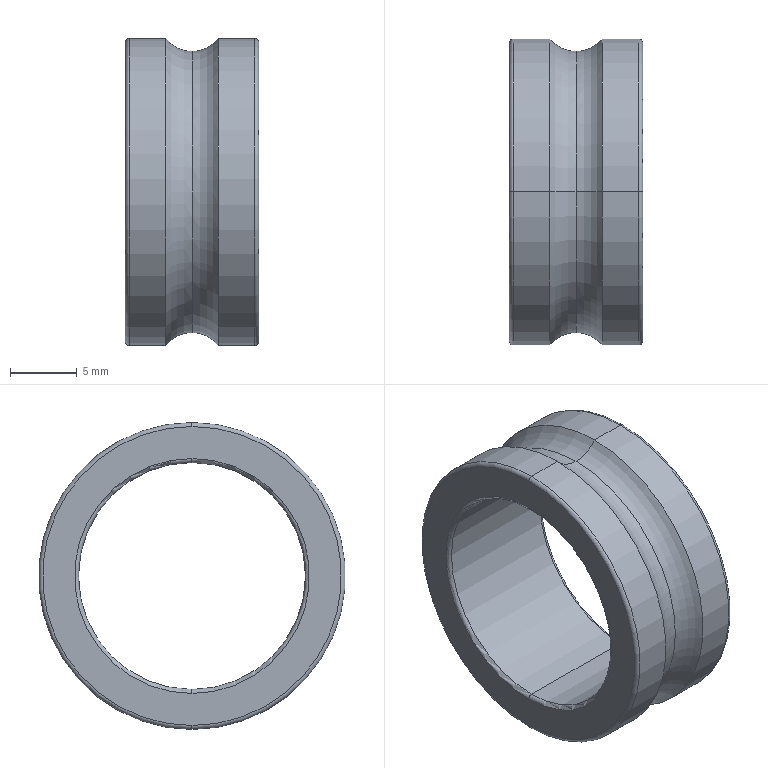Part | SolidWorks | features BaseBody 1 | 1 solid | 20 faces | box 10 x 23 x 23 mm | volume 1693 mm3 | torus 12 | cylinder 6 | plane 2 | commonest cylinder face diameters 23 x4 17 x2
STEP:
#1=CARTESIAN_POINT('',(-1.969,0.,11.5));
#2=VERTEX_POINT('',#1);
#3=CARTESIAN_POINT('',(0.,0.,10.525));
#4=VERTEX_POINT('',#3);
#5=CARTESIAN_POINT('',(0.,0.,13.));
#6=DIRECTION('',(0.,-1.,0.));
#7=DIRECTION('',(0.,0.,-1.));
#8=AXIS2_PLACEMENT_3D('',#5,#6,#7);
#9=CIRCLE('',#8,2.475);
#10=EDGE_CURVE('',#2,#4,#9,.T.);
#11=ORIENTED_EDGE('',*,*,#10,.T.);
#12=CARTESIAN_POINT('',(0.,0.,-10.525));
#13=VERTEX_POINT('',#12);
#14=CARTESIAN_POINT('',(0.,0.,0.));
#15=DIRECTION('',(-1.,0.,0.));
#16=DIRECTION('',(0.,0.,1.));
#17=AXIS2_PLACEMENT_3D('',#14,#15,#16);
#18=CIRCLE('',#17,10.525);
#19=EDGE_CURVE('',#4,#13,#18,.T.);
#20=ORIENTED_EDGE('',*,*,#19,.T.);
#21=CARTESIAN_POINT('',(-1.969,0.,-11.5));
#22=VERTEX_POINT('',#21);
#23=CARTESIAN_POINT('',(0.,0.,-13.));
#24=DIRECTION('',(0.,1.,0.));
#25=DIRECTION('',(0.,0.,1.));
#26=AXIS2_PLACEMENT_3D('',#23,#24,#25);
#27=CIRCLE('',#26,2.475);
#28=EDGE_CURVE('',#22,#13,#27,.T.);
#29=ORIENTED_EDGE('',*,*,#28,.F.);
#30=CARTESIAN_POINT('',(-1.969,0.,0.));
#31=DIRECTION('',(1.,0.,0.));
#32=DIRECTION('',(0.,0.,-1.));
#33=AXIS2_PLACEMENT_3D('',#30,#31,#32);
#34=CIRCLE('',#33,11.5);
#35=EDGE_CURVE('',#22,#2,#34,.T.);
#36=ORIENTED_EDGE('',*,*,#35,.T.);
#37=EDGE_LOOP('',(#11,#20,#29,#36));
#38=FACE_OUTER_BOUND('',#37,.T.);
#39=CARTESIAN_POINT('',(0.,0.,0.));
#40=DIRECTION('',(-1.,0.,0.));
#41=DIRECTION('',(0.,0.,1.));
#42=AXIS2_PLACEMENT_3D('',#39,#40,#41);
#43=TOROIDAL_SURFACE('',#42,13.,2.475);
#44=ADVANCED_FACE('',(#38),#43,.F.);
#45=ORIENTED_EDGE('',*,*,#28,.T.);
#46=CARTESIAN_POINT('',(0.,0.,0.));
#47=DIRECTION('',(-1.,0.,0.));
#48=DIRECTION('',(0.,0.,1.));
#49=AXIS2_PLACEMENT_3D('',#46,#47,#48);
#50=CIRCLE('',#49,10.525);
#51=EDGE_CURVE('',#13,#4,#50,.T.);
#52=ORIENTED_EDGE('',*,*,#51,.T.);
#53=ORIENTED_EDGE('',*,*,#10,.F.);
#54=CARTESIAN_POINT('',(-1.969,0.,0.));
#55=DIRECTION('',(1.,0.,0.));
#56=DIRECTION('',(0.,0.,-1.));
#57=AXIS2_PLACEMENT_3D('',#54,#55,#56);
#58=CIRCLE('',#57,11.5);
#59=EDGE_CURVE('',#2,#22,#58,.T.);
#60=ORIENTED_EDGE('',*,*,#59,.T.);
#61=EDGE_LOOP('',(#45,#52,#53,#60));
#62=FACE_OUTER_BOUND('',#61,.T.);
#63=CARTESIAN_POINT('',(0.,0.,0.));
#64=DIRECTION('',(-1.,0.,0.));
#65=DIRECTION('',(0.,0.,1.));
#66=AXIS2_PLACEMENT_3D('',#63,#64,#65);
#67=TOROIDAL_SURFACE('',#66,13.,2.475);
#68=ADVANCED_FACE('',(#62),#67,.F.);
#69=ORIENTED_EDGE('',*,*,#51,.F.);
#70=CARTESIAN_POINT('',(1.969,0.,-11.5));
#71=VERTEX_POINT('',#70);
#72=CARTESIAN_POINT('',(0.,0.,-13.));
#73=DIRECTION('',(0.,1.,0.));
#74=DIRECTION('',(0.,0.,1.));
#75=AXIS2_PLACEMENT_3D('',#72,#73,#74);
#76=CIRCLE('',#75,2.475);
#77=EDGE_CURVE('',#13,#71,#76,.T.);
#78=ORIENTED_EDGE('',*,*,#77,.T.);
#79=CARTESIAN_POINT('',(1.969,0.,11.5));
#80=VERTEX_POINT('',#79);
#81=CARTESIAN_POINT('',(1.969,0.,0.));
#82=DIRECTION('',(-1.,0.,0.));
#83=DIRECTION('',(0.,0.,1.));
#84=AXIS2_PLACEMENT_3D('',#81,#82,#83);
#85=CIRCLE('',#84,11.5);
#86=EDGE_CURVE('',#71,#80,#85,.T.);
#87=ORIENTED_EDGE('',*,*,#86,.T.);
#88=CARTESIAN_POINT('',(0.,0.,13.));
#89=DIRECTION('',(0.,-1.,0.));
#90=DIRECTION('',(0.,0.,-1.));
#91=AXIS2_PLACEMENT_3D('',#88,#89,#90);
#92=CIRCLE('',#91,2.475);
#93=EDGE_CURVE('',#4,#80,#92,.T.);
#94=ORIENTED_EDGE('',*,*,#93,.F.);
#95=EDGE_LOOP('',(#69,#78,#87,#94));
#96=FACE_OUTER_BOUND('',#95,.T.);
#97=CARTESIAN_POINT('',(0.,0.,0.));
#98=DIRECTION('',(-1.,0.,0.));
#99=DIRECTION('',(0.,0.,1.));
#100=AXIS2_PLACEMENT_3D('',#97,#98,#99);
#101=TOROIDAL_SURFACE('',#100,13.,2.475);
#102=ADVANCED_FACE('',(#96),#101,.F.);
#103=CARTESIAN_POINT('',(-4.7,0.,11.5));
#104=VERTEX_POINT('',#103);
#105=CARTESIAN_POINT('',(-4.7,0.,-11.5));
#106=VERTEX_POINT('',#105);
#107=CARTESIAN_POINT('',(-4.7,0.,0.));
#108=DIRECTION('',(-1.,0.,0.));
#109=DIRECTION('',(0.,0.,1.));
#110=AXIS2_PLACEMENT_3D('',#107,#108,#109);
#111=CIRCLE('',#110,11.5);
#112=EDGE_CURVE('',#104,#106,#111,.T.);
#113=ORIENTED_EDGE('',*,*,#112,.T.);
#114=CARTESIAN_POINT('',(-5.,0.,-11.2));
#115=VERTEX_POINT('',#114);
#116=CARTESIAN_POINT('',(-4.7,0.,-11.2));
#117=DIRECTION('',(0.,1.,0.));
#118=DIRECTION('',(0.,0.,1.));
#119=AXIS2_PLACEMENT_3D('',#116,#117,#118);
#120=CIRCLE('',#119,0.3);
#121=EDGE_CURVE('',#106,#115,#120,.T.);
#122=ORIENTED_EDGE('',*,*,#121,.T.);
#123=CARTESIAN_POINT('',(-5.,0.,11.2));
#124=VERTEX_POINT('',#123);
#125=CARTESIAN_POINT('',(-5.,0.,0.));
#126=DIRECTION('',(-1.,0.,0.));
#127=DIRECTION('',(0.,0.,1.));
#128=AXIS2_PLACEMENT_3D('',#125,#126,#127);
#129=CIRCLE('',#128,11.2);
#130=EDGE_CURVE('',#124,#115,#129,.T.);
#131=ORIENTED_EDGE('',*,*,#130,.F.);
#132=CARTESIAN_POINT('',(-4.7,0.,11.2));
#133=DIRECTION('',(0.,-1.,0.));
#134=DIRECTION('',(0.,0.,-1.));
#135=AXIS2_PLACEMENT_3D('',#132,#133,#134);
#136=CIRCLE('',#135,0.3);
#137=EDGE_CURVE('',#104,#124,#136,.T.);
#138=ORIENTED_EDGE('',*,*,#137,.F.);
#139=EDGE_LOOP('',(#113,#122,#131,#138));
#140=FACE_OUTER_BOUND('',#139,.T.);
#141=CARTESIAN_POINT('',(-4.7,0.,0.));
#142=DIRECTION('',(-1.,0.,0.));
#143=DIRECTION('',(0.,0.,1.));
#144=AXIS2_PLACEMENT_3D('',#141,#142,#143);
#145=TOROIDAL_SURFACE('',#144,11.2,0.3);
#146=ADVANCED_FACE('',(#140),#145,.T.);
#147=CARTESIAN_POINT('',(5.,0.,11.2));
#148=VERTEX_POINT('',#147);
#149=CARTESIAN_POINT('',(5.,0.,-11.2));
#150=VERTEX_POINT('',#149);
#151=CARTESIAN_POINT('',(5.,0.,0.));
#152=DIRECTION('',(-1.,0.,0.));
#153=DIRECTION('',(0.,0.,1.));
#154=AXIS2_PLACEMENT_3D('',#151,#152,#153);
#155=CIRCLE('',#154,11.2);
#156=EDGE_CURVE('',#148,#150,#155,.T.);
#157=ORIENTED_EDGE('',*,*,#156,.T.);
#158=CARTESIAN_POINT('',(4.7,0.,-11.5));
#159=VERTEX_POINT('',#158);
#160=CARTESIAN_POINT('',(4.7,0.,-11.2));
#161=DIRECTION('',(0.,1.,0.));
#162=DIRECTION('',(0.,0.,1.));
#163=AXIS2_PLACEMENT_3D('',#160,#161,#162);
#164=CIRCLE('',#163,0.3);
#165=EDGE_CURVE('',#150,#159,#164,.T.);
#166=ORIENTED_EDGE('',*,*,#165,.T.);
#167=CARTESIAN_POINT('',(4.7,0.,11.5));
#168=VERTEX_POINT('',#167);
#169=CARTESIAN_POINT('',(4.7,0.,0.));
#170=DIRECTION('',(-1.,0.,0.));
#171=DIRECTION('',(0.,0.,1.));
#172=AXIS2_PLACEMENT_3D('',#169,#170,#171);
#173=CIRCLE('',#172,11.5);
#174=EDGE_CURVE('',#168,#159,#173,.T.);
#175=ORIENTED_EDGE('',*,*,#174,.F.);
#176=CARTESIAN_POINT('',(4.7,0.,11.2));
#177=DIRECTION('',(0.,-1.,0.));
#178=DIRECTION('',(0.,0.,-1.));
#179=AXIS2_PLACEMENT_3D('',#176,#177,#178);
#180=CIRCLE('',#179,0.3);
#181=EDGE_CURVE('',#148,#168,#180,.T.);
#182=ORIENTED_EDGE('',*,*,#181,.F.);
#183=EDGE_LOOP('',(#157,#166,#175,#182));
#184=FACE_OUTER_BOUND('',#183,.T.);
#185=CARTESIAN_POINT('',(4.7,0.,0.));
#186=DIRECTION('',(-1.,0.,0.));
#187=DIRECTION('',(0.,0.,1.));
#188=AXIS2_PLACEMENT_3D('',#185,#186,#187);
#189=TOROIDAL_SURFACE('',#188,11.2,0.3);
#190=ADVANCED_FACE('',(#184),#189,.T.);
#191=CARTESIAN_POINT('',(4.7,0.,8.5));
#192=VERTEX_POINT('',#191);
#193=CARTESIAN_POINT('',(4.7,0.,-8.5));
#194=VERTEX_POINT('',#193);
#195=CARTESIAN_POINT('',(4.7,0.,0.));
#196=DIRECTION('',(-1.,0.,0.));
#197=DIRECTION('',(0.,0.,1.));
#198=AXIS2_PLACEMENT_3D('',#195,#196,#197);
#199=CIRCLE('',#198,8.5);
#200=EDGE_CURVE('',#192,#194,#199,.T.);
#201=ORIENTED_EDGE('',*,*,#200,.T.);
#202=CARTESIAN_POINT('',(5.,0.,-8.8));
#203=VERTEX_POINT('',#202);
#204=CARTESIAN_POINT('',(4.7,0.,-8.8));
#205=DIRECTION('',(0.,1.,0.));
#206=DIRECTION('',(0.,0.,1.));
#207=AXIS2_PLACEMENT_3D('',#204,#205,#206);
#208=CIRCLE('',#207,0.3);
#209=EDGE_CURVE('',#194,#203,#208,.T.);
#210=ORIENTED_EDGE('',*,*,#209,.T.);
#211=CARTESIAN_POINT('',(5.,0.,8.8));
#212=VERTEX_POINT('',#211);
#213=CARTESIAN_POINT('',(5.,0.,0.));
#214=DIRECTION('',(-1.,0.,0.));
#215=DIRECTION('',(0.,0.,1.));
#216=AXIS2_PLACEMENT_3D('',#213,#214,#215);
#217=CIRCLE('',#216,8.8);
#218=EDGE_CURVE('',#212,#203,#217,.T.);
#219=ORIENTED_EDGE('',*,*,#218,.F.);
#220=CARTESIAN_POINT('',(4.7,0.,8.8));
#221=DIRECTION('',(0.,-1.,0.));
#222=DIRECTION('',(0.,0.,-1.));
#223=AXIS2_PLACEMENT_3D('',#220,#221,#222);
#224=CIRCLE('',#223,0.3);
#225=EDGE_CURVE('',#192,#212,#224,.T.);
#226=ORIENTED_EDGE('',*,*,#225,.F.);
#227=EDGE_LOOP('',(#201,#210,#219,#226));
#228=FACE_OUTER_BOUND('',#227,.T.);
#229=CARTESIAN_POINT('',(4.7,0.,0.));
#230=DIRECTION('',(-1.,0.,0.));
#231=DIRECTION('',(0.,0.,1.));
#232=AXIS2_PLACEMENT_3D('',#229,#230,#231);
#233=TOROIDAL_SURFACE('',#232,8.8,0.3);
#234=ADVANCED_FACE('',(#228),#233,.T.);
#235=CARTESIAN_POINT('',(4.7,0.,0.));
#236=DIRECTION('',(-1.,0.,0.));
#237=DIRECTION('',(0.,0.,1.));
#238=AXIS2_PLACEMENT_3D('',#235,#236,#237);
#239=CIRCLE('',#238,8.5);
#240=EDGE_CURVE('',#194,#192,#239,.T.);
#241=ORIENTED_EDGE('',*,*,#240,.F.);
#242=CARTESIAN_POINT('',(-4.7,0.,-8.5));
#243=VERTEX_POINT('',#242);
#244=CARTESIAN_POINT('',(-3.5,0.,-8.5));
#245=DIRECTION('',(-1.,0.,0.));
#246=VECTOR('',#245,1000.);
#247=LINE('',#244,#246);
#248=EDGE_CURVE('',#194,#243,#247,.T.);
#249=ORIENTED_EDGE('',*,*,#248,.T.);
#250=CARTESIAN_POINT('',(-4.7,0.,8.5));
#251=VERTEX_POINT('',#250);
#252=CARTESIAN_POINT('',(-4.7,0.,0.));
#253=DIRECTION('',(-1.,0.,0.));
#254=DIRECTION('',(0.,0.,1.));
#255=AXIS2_PLACEMENT_3D('',#252,#253,#254);
#256=CIRCLE('',#255,8.5);
#257=EDGE_CURVE('',#243,#251,#256,.T.);
#258=ORIENTED_EDGE('',*,*,#257,.T.);
#259=CARTESIAN_POINT('',(-3.5,0.,8.5));
#260=DIRECTION('',(-1.,0.,0.));
#261=VECTOR('',#260,1000.);
#262=LINE('',#259,#261);
#263=EDGE_CURVE('',#192,#251,#262,.T.);
#264=ORIENTED_EDGE('',*,*,#263,.F.);
#265=EDGE_LOOP('',(#241,#249,#258,#264));
#266=FACE_OUTER_BOUND('',#265,.T.);
#267=CARTESIAN_POINT('',(-3.5,0.,0.));
#268=DIRECTION('',(-1.,0.,0.));
#269=DIRECTION('',(0.,0.,1.));
#270=AXIS2_PLACEMENT_3D('',#267,#268,#269);
#271=CYLINDRICAL_SURFACE('',#270,8.5);
#272=ADVANCED_FACE('',(#266),#271,.F.);
#273=CARTESIAN_POINT('',(-5.,0.,8.8));
#274=VERTEX_POINT('',#273);
#275=CARTESIAN_POINT('',(-5.,0.,-8.8));
#276=VERTEX_POINT('',#275);
#277=CARTESIAN_POINT('',(-5.,0.,0.));
#278=DIRECTION('',(-1.,0.,0.));
#279=DIRECTION('',(0.,0.,1.));
#280=AXIS2_PLACEMENT_3D('',#277,#278,#279);
#281=CIRCLE('',#280,8.8);
#282=EDGE_CURVE('',#274,#276,#281,.T.);
#283=ORIENTED_EDGE('',*,*,#282,.T.);
#284=CARTESIAN_POINT('',(-4.7,0.,-8.8));
#285=DIRECTION('',(0.,1.,0.));
#286=DIRECTION('',(0.,0.,1.));
#287=AXIS2_PLACEMENT_3D('',#284,#285,#286);
#288=CIRCLE('',#287,0.3);
#289=EDGE_CURVE('',#276,#243,#288,.T.);
#290=ORIENTED_EDGE('',*,*,#289,.T.);
#291=CARTESIAN_POINT('',(-4.7,0.,0.));
#292=DIRECTION('',(-1.,0.,0.));
#293=DIRECTION('',(0.,0.,1.));
#294=AXIS2_PLACEMENT_3D('',#291,#292,#293);
#295=CIRCLE('',#294,8.5);
#296=EDGE_CURVE('',#251,#243,#295,.T.);
#297=ORIENTED_EDGE('',*,*,#296,.F.);
#298=CARTESIAN_POINT('',(-4.7,0.,8.8));
#299=DIRECTION('',(0.,-1.,0.));
#300=DIRECTION('',(0.,0.,-1.));
#301=AXIS2_PLACEMENT_3D('',#298,#299,#300);
#302=CIRCLE('',#301,0.3);
#303=EDGE_CURVE('',#274,#251,#302,.T.);
#304=ORIENTED_EDGE('',*,*,#303,.F.);
#305=EDGE_LOOP('',(#283,#290,#297,#304));
#306=FACE_OUTER_BOUND('',#305,.T.);
#307=CARTESIAN_POINT('',(-4.7,0.,0.));
#308=DIRECTION('',(-1.,0.,0.));
#309=DIRECTION('',(0.,0.,1.));
#310=AXIS2_PLACEMENT_3D('',#307,#308,#309);
#311=TOROIDAL_SURFACE('',#310,8.8,0.3);
#312=ADVANCED_FACE('',(#306),#311,.T.);
#313=ORIENTED_EDGE('',*,*,#35,.F.);
#314=CARTESIAN_POINT('',(-3.5,0.,-11.5));
#315=DIRECTION('',(-1.,0.,0.));
#316=VECTOR('',#315,1000.);
#317=LINE('',#314,#316);
#318=EDGE_CURVE('',#22,#106,#317,.T.);
#319=ORIENTED_EDGE('',*,*,#318,.T.);
#320=ORIENTED_EDGE('',*,*,#112,.F.);
#321=CARTESIAN_POINT('',(-3.5,0.,11.5));
#322=DIRECTION('',(-1.,0.,0.));
#323=VECTOR('',#322,1000.);
#324=LINE('',#321,#323);
#325=EDGE_CURVE('',#2,#104,#324,.T.);
#326=ORIENTED_EDGE('',*,*,#325,.F.);
#327=EDGE_LOOP('',(#313,#319,#320,#326));
#328=FACE_OUTER_BOUND('',#327,.T.);
#329=CARTESIAN_POINT('',(-3.5,0.,0.));
#330=DIRECTION('',(-1.,0.,0.));
#331=DIRECTION('',(0.,0.,1.));
#332=AXIS2_PLACEMENT_3D('',#329,#330,#331);
#333=CYLINDRICAL_SURFACE('',#332,11.5);
#334=ADVANCED_FACE('',(#328),#333,.T.);
#335=ORIENTED_EDGE('',*,*,#174,.T.);
#336=CARTESIAN_POINT('',(-3.5,0.,-11.5));
#337=DIRECTION('',(-1.,0.,0.));
#338=VECTOR('',#337,1000.);
#339=LINE('',#336,#338);
#340=EDGE_CURVE('',#159,#71,#339,.T.);
#341=ORIENTED_EDGE('',*,*,#340,.T.);
#342=CARTESIAN_POINT('',(1.969,0.,0.));
#343=DIRECTION('',(-1.,0.,0.));
#344=DIRECTION('',(0.,0.,1.));
#345=AXIS2_PLACEMENT_3D('',#342,#343,#344);
#346=CIRCLE('',#345,11.5);
#347=EDGE_CURVE('',#80,#71,#346,.T.);
#348=ORIENTED_EDGE('',*,*,#347,.F.);
#349=CARTESIAN_POINT('',(-3.5,0.,11.5));
#350=DIRECTION('',(-1.,0.,0.));
#351=VECTOR('',#350,1000.);
#352=LINE('',#349,#351);
#353=EDGE_CURVE('',#168,#80,#352,.T.);
#354=ORIENTED_EDGE('',*,*,#353,.F.);
#355=EDGE_LOOP('',(#335,#341,#348,#354));
#356=FACE_OUTER_BOUND('',#355,.T.);
#357=CARTESIAN_POINT('',(-3.5,0.,0.));
#358=DIRECTION('',(-1.,0.,0.));
#359=DIRECTION('',(0.,0.,1.));
#360=AXIS2_PLACEMENT_3D('',#357,#358,#359);
#361=CYLINDRICAL_SURFACE('',#360,11.5);
#362=ADVANCED_FACE('',(#356),#361,.T.);
#363=ORIENTED_EDGE('',*,*,#282,.F.);
#364=CARTESIAN_POINT('',(-5.,0.,0.));
#365=DIRECTION('',(-1.,0.,0.));
#366=DIRECTION('',(0.,0.,1.));
#367=AXIS2_PLACEMENT_3D('',#364,#365,#366);
#368=CIRCLE('',#367,8.8);
#369=EDGE_CURVE('',#276,#274,#368,.T.);
#370=ORIENTED_EDGE('',*,*,#369,.F.);
#371=EDGE_LOOP('',(#363,#370));
#372=FACE_BOUND('',#371,.T.);
#373=ORIENTED_EDGE('',*,*,#130,.T.);
#374=CARTESIAN_POINT('',(-5.,0.,0.));
#375=DIRECTION('',(-1.,0.,0.));
#376=DIRECTION('',(0.,0.,1.));
#377=AXIS2_PLACEMENT_3D('',#374,#375,#376);
#378=CIRCLE('',#377,11.2);
#379=EDGE_CURVE('',#115,#124,#378,.T.);
#380=ORIENTED_EDGE('',*,*,#379,.T.);
#381=EDGE_LOOP('',(#373,#380));
#382=FACE_OUTER_BOUND('',#381,.T.);
#383=CARTESIAN_POINT('',(-5.,8.8,0.));
#384=DIRECTION('',(1.,0.,0.));
#385=DIRECTION('',(0.,1.,0.));
#386=AXIS2_PLACEMENT_3D('',#383,#384,#385);
#387=PLANE('',#386);
#388=ADVANCED_FACE('',(#372,#382),#387,.F.);
#389=ORIENTED_EDGE('',*,*,#218,.T.);
#390=CARTESIAN_POINT('',(5.,0.,0.));
#391=DIRECTION('',(-1.,0.,0.));
#392=DIRECTION('',(0.,0.,1.));
#393=AXIS2_PLACEMENT_3D('',#390,#391,#392);
#394=CIRCLE('',#393,8.8);
#395=EDGE_CURVE('',#203,#212,#394,.T.);
#396=ORIENTED_EDGE('',*,*,#395,.T.);
#397=EDGE_LOOP('',(#389,#396));
#398=FACE_BOUND('',#397,.T.);
#399=ORIENTED_EDGE('',*,*,#156,.F.);
#400=CARTESIAN_POINT('',(5.,0.,0.));
#401=DIRECTION('',(-1.,0.,0.));
#402=DIRECTION('',(0.,0.,1.));
#403=AXIS2_PLACEMENT_3D('',#400,#401,#402);
#404=CIRCLE('',#403,11.2);
#405=EDGE_CURVE('',#150,#148,#404,.T.);
#406=ORIENTED_EDGE('',*,*,#405,.F.);
#407=EDGE_LOOP('',(#399,#406));
#408=FACE_OUTER_BOUND('',#407,.T.);
#409=CARTESIAN_POINT('',(5.,11.2,0.));
#410=DIRECTION('',(-1.,0.,0.));
#411=DIRECTION('',(0.,0.,1.));
#412=AXIS2_PLACEMENT_3D('',#409,#410,#411);
#413=PLANE('',#412);
#414=ADVANCED_FACE('',(#398,#408),#413,.F.);
#415=ORIENTED_EDGE('',*,*,#340,.F.);
#416=CARTESIAN_POINT('',(4.7,0.,0.));
#417=DIRECTION('',(-1.,0.,0.));
#418=DIRECTION('',(0.,0.,1.));
#419=AXIS2_PLACEMENT_3D('',#416,#417,#418);
#420=CIRCLE('',#419,11.5);
#421=EDGE_CURVE('',#159,#168,#420,.T.);
#422=ORIENTED_EDGE('',*,*,#421,.T.);
#423=ORIENTED_EDGE('',*,*,#353,.T.);
#424=ORIENTED_EDGE('',*,*,#86,.F.);
#425=EDGE_LOOP('',(#415,#422,#423,#424));
#426=FACE_OUTER_BOUND('',#425,.T.);
#427=CARTESIAN_POINT('',(-3.5,0.,0.));
#428=DIRECTION('',(-1.,0.,0.));
#429=DIRECTION('',(0.,0.,1.));
#430=AXIS2_PLACEMENT_3D('',#427,#428,#429);
#431=CYLINDRICAL_SURFACE('',#430,11.5);
#432=ADVANCED_FACE('',(#426),#431,.T.);
#433=ORIENTED_EDGE('',*,*,#318,.F.);
#434=ORIENTED_EDGE('',*,*,#59,.F.);
#435=ORIENTED_EDGE('',*,*,#325,.T.);
#436=CARTESIAN_POINT('',(-4.7,0.,0.));
#437=DIRECTION('',(-1.,0.,0.));
#438=DIRECTION('',(0.,0.,1.));
#439=AXIS2_PLACEMENT_3D('',#436,#437,#438);
#440=CIRCLE('',#439,11.5);
#441=EDGE_CURVE('',#106,#104,#440,.T.);
#442=ORIENTED_EDGE('',*,*,#441,.F.);
#443=EDGE_LOOP('',(#433,#434,#435,#442));
#444=FACE_OUTER_BOUND('',#443,.T.);
#445=CARTESIAN_POINT('',(-3.5,0.,0.));
#446=DIRECTION('',(-1.,0.,0.));
#447=DIRECTION('',(0.,0.,1.));
#448=AXIS2_PLACEMENT_3D('',#445,#446,#447);
#449=CYLINDRICAL_SURFACE('',#448,11.5);
#450=ADVANCED_FACE('',(#444),#449,.T.);
#451=ORIENTED_EDGE('',*,*,#289,.F.);
#452=ORIENTED_EDGE('',*,*,#369,.T.);
#453=ORIENTED_EDGE('',*,*,#303,.T.);
#454=ORIENTED_EDGE('',*,*,#257,.F.);
#455=EDGE_LOOP('',(#451,#452,#453,#454));
#456=FACE_OUTER_BOUND('',#455,.T.);
#457=CARTESIAN_POINT('',(-4.7,0.,0.));
#458=DIRECTION('',(-1.,0.,0.));
#459=DIRECTION('',(0.,0.,1.));
#460=AXIS2_PLACEMENT_3D('',#457,#458,#459);
#461=TOROIDAL_SURFACE('',#460,8.8,0.3);
#462=ADVANCED_FACE('',(#456),#461,.T.);
#463=ORIENTED_EDGE('',*,*,#248,.F.);
#464=ORIENTED_EDGE('',*,*,#200,.F.);
#465=ORIENTED_EDGE('',*,*,#263,.T.);
#466=ORIENTED_EDGE('',*,*,#296,.T.);
#467=EDGE_LOOP('',(#463,#464,#465,#466));
#468=FACE_OUTER_BOUND('',#467,.T.);
#469=CARTESIAN_POINT('',(-3.5,0.,0.));
#470=DIRECTION('',(-1.,0.,0.));
#471=DIRECTION('',(0.,0.,1.));
#472=AXIS2_PLACEMENT_3D('',#469,#470,#471);
#473=CYLINDRICAL_SURFACE('',#472,8.5);
#474=ADVANCED_FACE('',(#468),#473,.F.);
#475=ORIENTED_EDGE('',*,*,#209,.F.);
#476=ORIENTED_EDGE('',*,*,#240,.T.);
#477=ORIENTED_EDGE('',*,*,#225,.T.);
#478=ORIENTED_EDGE('',*,*,#395,.F.);
#479=EDGE_LOOP('',(#475,#476,#477,#478));
#480=FACE_OUTER_BOUND('',#479,.T.);
#481=CARTESIAN_POINT('',(4.7,0.,0.));
#482=DIRECTION('',(-1.,0.,0.));
#483=DIRECTION('',(0.,0.,1.));
#484=AXIS2_PLACEMENT_3D('',#481,#482,#483);
#485=TOROIDAL_SURFACE('',#484,8.8,0.3);
#486=ADVANCED_FACE('',(#480),#485,.T.);
#487=ORIENTED_EDGE('',*,*,#165,.F.);
#488=ORIENTED_EDGE('',*,*,#405,.T.);
#489=ORIENTED_EDGE('',*,*,#181,.T.);
#490=ORIENTED_EDGE('',*,*,#421,.F.);
#491=EDGE_LOOP('',(#487,#488,#489,#490));
#492=FACE_OUTER_BOUND('',#491,.T.);
#493=CARTESIAN_POINT('',(4.7,0.,0.));
#494=DIRECTION('',(-1.,0.,0.));
#495=DIRECTION('',(0.,0.,1.));
#496=AXIS2_PLACEMENT_3D('',#493,#494,#495);
#497=TOROIDAL_SURFACE('',#496,11.2,0.3);
#498=ADVANCED_FACE('',(#492),#497,.T.);
#499=ORIENTED_EDGE('',*,*,#121,.F.);
#500=ORIENTED_EDGE('',*,*,#441,.T.);
#501=ORIENTED_EDGE('',*,*,#137,.T.);
#502=ORIENTED_EDGE('',*,*,#379,.F.);
#503=EDGE_LOOP('',(#499,#500,#501,#502));
#504=FACE_OUTER_BOUND('',#503,.T.);
#505=CARTESIAN_POINT('',(-4.7,0.,0.));
#506=DIRECTION('',(-1.,0.,0.));
#507=DIRECTION('',(0.,0.,1.));
#508=AXIS2_PLACEMENT_3D('',#505,#506,#507);
#509=TOROIDAL_SURFACE('',#508,11.2,0.3);
#510=ADVANCED_FACE('',(#504),#509,.T.);
#511=ORIENTED_EDGE('',*,*,#19,.F.);
#512=ORIENTED_EDGE('',*,*,#93,.T.);
#513=ORIENTED_EDGE('',*,*,#347,.T.);
#514=ORIENTED_EDGE('',*,*,#77,.F.);
#515=EDGE_LOOP('',(#511,#512,#513,#514));
#516=FACE_OUTER_BOUND('',#515,.T.);
#517=CARTESIAN_POINT('',(0.,0.,0.));
#518=DIRECTION('',(-1.,0.,0.));
#519=DIRECTION('',(0.,0.,1.));
#520=AXIS2_PLACEMENT_3D('',#517,#518,#519);
#521=TOROIDAL_SURFACE('',#520,13.,2.475);
#522=ADVANCED_FACE('',(#516),#521,.F.);
#523=CLOSED_SHELL('',(#44,#68,#102,#146,#190,#234,#272,#312,#334,#362,#388,#414,#432,#450,#462,#474,#486,#498,#510,#522));
#524=MANIFOLD_SOLID_BREP('',#523);
#525=CARTESIAN_POINT('',(0.,0.,0.));
#526=DIRECTION('',(0.,0.,1.));
#527=DIRECTION('',(1.,0.,0.));
#528=AXIS2_PLACEMENT_3D('',#525,#526,#527);
#529=(LENGTH_UNIT()NAMED_UNIT(*)SI_UNIT(.MILLI.,.METRE.));
#530=UNCERTAINTY_MEASURE_WITH_UNIT(LENGTH_MEASURE(0.00001),#529,'','');
#531=(NAMED_UNIT(*)PLANE_ANGLE_UNIT()SI_UNIT($,.RADIAN.));
#532=(NAMED_UNIT(*)SI_UNIT($,.STERADIAN.)SOLID_ANGLE_UNIT());
#533=(GEOMETRIC_REPRESENTATION_CONTEXT(3)GLOBAL_UNCERTAINTY_ASSIGNED_CONTEXT((#530))GLOBAL_UNIT_ASSIGNED_CONTEXT((#529,#531,#532))REPRESENTATION_CONTEXT('',''));
#534=ADVANCED_BREP_SHAPE_REPRESENTATION('',(#524,#528),#533);